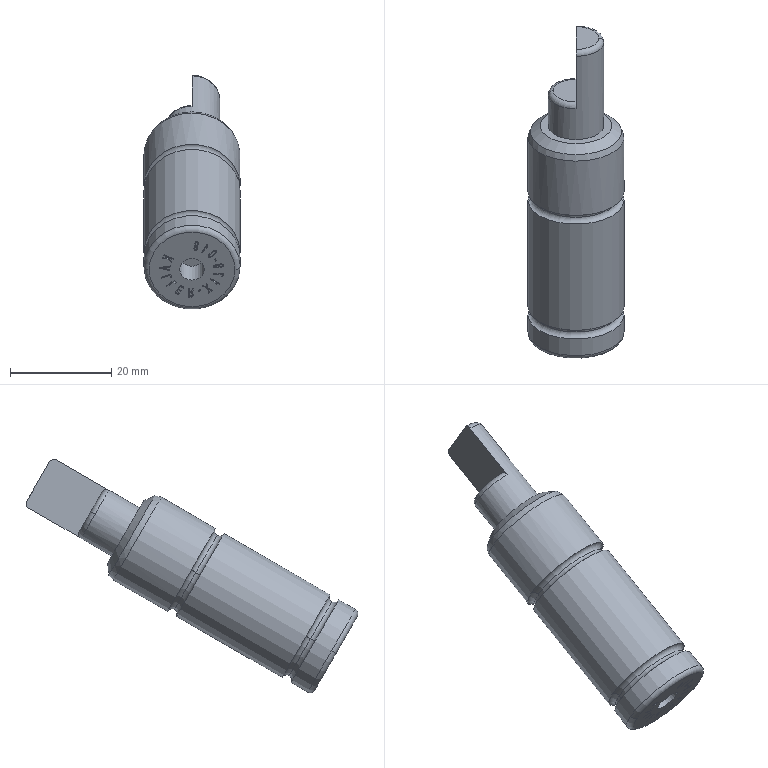Part | NX | features 1 2 | 1 solid | 162 faces | box 19 x 65.657 x 46.26 mm | volume 14513 mm3 | plane 110 | spline 31 | torus 14 | cylinder 5 | cone 2 | commonest cylinder face diameters 19 x3 4.9 x1 11 x1